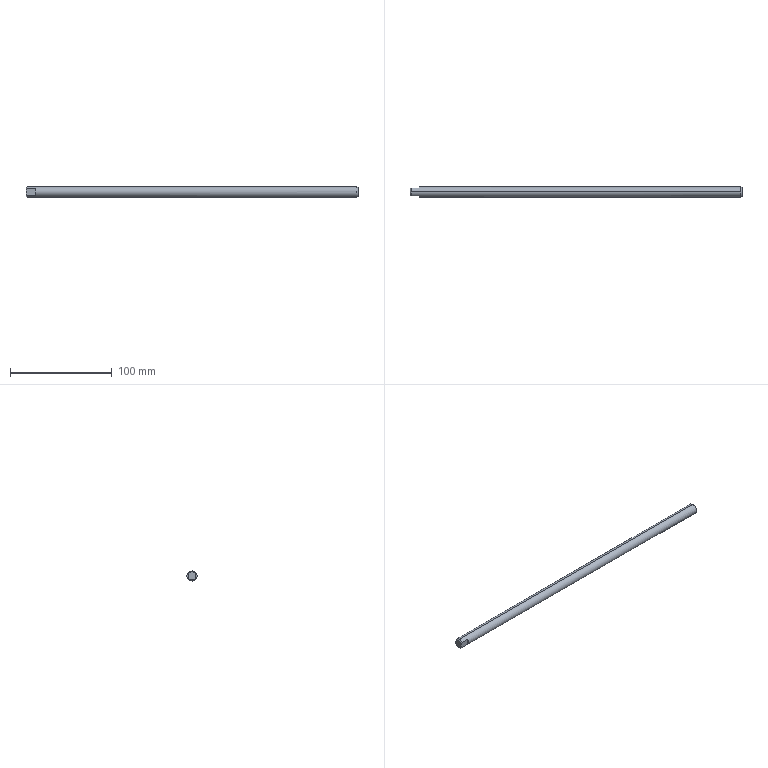Part | SolidWorks | features HoleWzd 2, Chamfer 1, Extrusion 1, ICE 1 | 1 solid | 13 faces | box 326 x 10 x 10 mm | volume 25495 mm3 | plane 6 | cone 5 | cylinder 2 | commonest cylinder face diameters 10 x2
STEP:
#1=CARTESIAN_POINT('',(326.,0.,-4.));
#2=VERTEX_POINT('',#1);
#3=CARTESIAN_POINT('',(326.,0.,4.));
#4=VERTEX_POINT('',#3);
#5=CARTESIAN_POINT('',(326.,0.,0.));
#6=DIRECTION('',(1.,0.,0.));
#7=DIRECTION('',(0.,0.,-1.));
#8=AXIS2_PLACEMENT_3D('',#5,#6,#7);
#9=CIRCLE('',#8,4.);
#10=EDGE_CURVE('',#2,#4,#9,.T.);
#11=ORIENTED_EDGE('',*,*,#10,.F.);
#12=CARTESIAN_POINT('',(325.,0.,-5.));
#13=VERTEX_POINT('',#12);
#14=CARTESIAN_POINT('',(326.,0.,-4.));
#15=DIRECTION('',(-0.7071,0.,-0.7071));
#16=VECTOR('',#15,1000.);
#17=LINE('',#14,#16);
#18=EDGE_CURVE('',#2,#13,#17,.T.);
#19=ORIENTED_EDGE('',*,*,#18,.T.);
#20=CARTESIAN_POINT('',(325.,0.,5.));
#21=VERTEX_POINT('',#20);
#22=CARTESIAN_POINT('',(325.,0.,0.));
#23=DIRECTION('',(-1.,0.,0.));
#24=DIRECTION('',(0.,0.,-1.));
#25=AXIS2_PLACEMENT_3D('',#22,#23,#24);
#26=CIRCLE('',#25,5.);
#27=EDGE_CURVE('',#21,#13,#26,.T.);
#28=ORIENTED_EDGE('',*,*,#27,.F.);
#29=CARTESIAN_POINT('',(326.,0.,4.));
#30=DIRECTION('',(-0.7071,0.,0.7071));
#31=VECTOR('',#30,1000.);
#32=LINE('',#29,#31);
#33=EDGE_CURVE('',#4,#21,#32,.T.);
#34=ORIENTED_EDGE('',*,*,#33,.F.);
#35=EDGE_LOOP('',(#11,#19,#28,#34));
#36=FACE_OUTER_BOUND('',#35,.T.);
#37=CARTESIAN_POINT('',(326.,0.,0.));
#38=DIRECTION('',(-1.,0.,0.));
#39=DIRECTION('',(0.,0.,1.));
#40=AXIS2_PLACEMENT_3D('',#37,#38,#39);
#41=CONICAL_SURFACE('',#40,4.,0.7854);
#42=ADVANCED_FACE('',(#36),#41,.T.);
#43=ORIENTED_EDGE('',*,*,#27,.T.);
#44=CARTESIAN_POINT('',(1.,0.,-5.));
#45=VERTEX_POINT('',#44);
#46=CARTESIAN_POINT('',(326.,0.,-5.));
#47=DIRECTION('',(-1.,0.,0.));
#48=VECTOR('',#47,1000.);
#49=LINE('',#46,#48);
#50=EDGE_CURVE('',#13,#45,#49,.T.);
#51=ORIENTED_EDGE('',*,*,#50,.T.);
#52=CARTESIAN_POINT('',(1.,3.9,-3.129));
#53=VERTEX_POINT('',#52);
#54=CARTESIAN_POINT('',(1.,0.,0.));
#55=DIRECTION('',(1.,0.,0.));
#56=DIRECTION('',(0.,0.,-1.));
#57=AXIS2_PLACEMENT_3D('',#54,#55,#56);
#58=CIRCLE('',#57,5.);
#59=EDGE_CURVE('',#45,#53,#58,.T.);
#60=ORIENTED_EDGE('',*,*,#59,.T.);
#61=CARTESIAN_POINT('',(9.,3.9,-3.129));
#62=VERTEX_POINT('',#61);
#63=CARTESIAN_POINT('',(326.,3.9,-3.129));
#64=DIRECTION('',(1.,0.,0.));
#65=VECTOR('',#64,1000.);
#66=LINE('',#63,#65);
#67=EDGE_CURVE('',#53,#62,#66,.T.);
#68=ORIENTED_EDGE('',*,*,#67,.T.);
#69=CARTESIAN_POINT('',(9.,3.9,3.129));
#70=VERTEX_POINT('',#69);
#71=CARTESIAN_POINT('',(9.,0.,0.));
#72=DIRECTION('',(1.,0.,0.));
#73=DIRECTION('',(0.,1.,0.));
#74=AXIS2_PLACEMENT_3D('',#71,#72,#73);
#75=CIRCLE('',#74,5.);
#76=EDGE_CURVE('',#62,#70,#75,.T.);
#77=ORIENTED_EDGE('',*,*,#76,.T.);
#78=CARTESIAN_POINT('',(1.,3.9,3.129));
#79=VERTEX_POINT('',#78);
#80=CARTESIAN_POINT('',(326.,3.9,3.129));
#81=DIRECTION('',(-1.,0.,0.));
#82=VECTOR('',#81,1000.);
#83=LINE('',#80,#82);
#84=EDGE_CURVE('',#70,#79,#83,.T.);
#85=ORIENTED_EDGE('',*,*,#84,.T.);
#86=CARTESIAN_POINT('',(1.,0.,5.));
#87=VERTEX_POINT('',#86);
#88=CARTESIAN_POINT('',(1.,0.,0.));
#89=DIRECTION('',(1.,0.,0.));
#90=DIRECTION('',(0.,0.,-1.));
#91=AXIS2_PLACEMENT_3D('',#88,#89,#90);
#92=CIRCLE('',#91,5.);
#93=EDGE_CURVE('',#79,#87,#92,.T.);
#94=ORIENTED_EDGE('',*,*,#93,.T.);
#95=CARTESIAN_POINT('',(326.,0.,5.));
#96=DIRECTION('',(-1.,0.,0.));
#97=VECTOR('',#96,1000.);
#98=LINE('',#95,#97);
#99=EDGE_CURVE('',#21,#87,#98,.T.);
#100=ORIENTED_EDGE('',*,*,#99,.F.);
#101=EDGE_LOOP('',(#43,#51,#60,#68,#77,#85,#94,#100));
#102=FACE_OUTER_BOUND('',#101,.T.);
#103=CARTESIAN_POINT('',(326.,0.,0.));
#104=DIRECTION('',(-1.,0.,0.));
#105=DIRECTION('',(0.,0.,1.));
#106=AXIS2_PLACEMENT_3D('',#103,#104,#105);
#107=CYLINDRICAL_SURFACE('',#106,5.);
#108=ADVANCED_FACE('',(#102),#107,.T.);
#109=CARTESIAN_POINT('',(0.,0.,-4.));
#110=VERTEX_POINT('',#109);
#111=CARTESIAN_POINT('',(0.,-3.9,-0.8888));
#112=VERTEX_POINT('',#111);
#113=CARTESIAN_POINT('',(0.,0.,0.));
#114=DIRECTION('',(-1.,0.,0.));
#115=DIRECTION('',(0.,0.,-1.));
#116=AXIS2_PLACEMENT_3D('',#113,#114,#115);
#117=CIRCLE('',#116,4.);
#118=EDGE_CURVE('',#110,#112,#117,.T.);
#119=ORIENTED_EDGE('',*,*,#118,.F.);
#120=CARTESIAN_POINT('',(1.,0.,-5.));
#121=DIRECTION('',(0.7071,0.,-0.7071));
#122=VECTOR('',#121,1000.);
#123=LINE('',#120,#122);
#124=EDGE_CURVE('',#110,#45,#123,.T.);
#125=ORIENTED_EDGE('',*,*,#124,.T.);
#126=CARTESIAN_POINT('',(1.,-3.9,-3.129));
#127=VERTEX_POINT('',#126);
#128=CARTESIAN_POINT('',(1.,0.,0.));
#129=DIRECTION('',(1.,0.,0.));
#130=DIRECTION('',(0.,0.,-1.));
#131=AXIS2_PLACEMENT_3D('',#128,#129,#130);
#132=CIRCLE('',#131,5.);
#133=EDGE_CURVE('',#127,#45,#132,.T.);
#134=ORIENTED_EDGE('',*,*,#133,.F.);
#135=CARTESIAN_POINT('',(0.,-3.9,-0.8888));
#136=CARTESIAN_POINT('',(0.0892,-3.9,-1.29));
#137=CARTESIAN_POINT('',(0.2351,-3.9,-1.683));
#138=CARTESIAN_POINT('',(0.5817,-3.9,-2.427));
#139=CARTESIAN_POINT('',(0.7831,-3.9,-2.782));
#140=CARTESIAN_POINT('',(1.,-3.9,-3.129));
#141=B_SPLINE_CURVE_WITH_KNOTS('',3,(#135,#136,#137,#138,#139,#140),.UNSPECIFIED.,.F.,.F.,(4,2,4),(0.01365,0.01489,0.01613),.UNSPECIFIED.);
#142=EDGE_CURVE('',#112,#127,#141,.T.);
#143=ORIENTED_EDGE('',*,*,#142,.F.);
#144=EDGE_LOOP('',(#119,#125,#134,#143));
#145=FACE_OUTER_BOUND('',#144,.T.);
#146=CARTESIAN_POINT('',(1.,0.,0.));
#147=DIRECTION('',(1.,0.,0.));
#148=DIRECTION('',(0.,0.,-1.));
#149=AXIS2_PLACEMENT_3D('',#146,#147,#148);
#150=CONICAL_SURFACE('',#149,5.,0.7854);
#151=ADVANCED_FACE('',(#145),#150,.T.);
#152=ORIENTED_EDGE('',*,*,#124,.F.);
#153=CARTESIAN_POINT('',(0.,3.9,-0.8888));
#154=VERTEX_POINT('',#153);
#155=CARTESIAN_POINT('',(0.,0.,0.));
#156=DIRECTION('',(-1.,0.,0.));
#157=DIRECTION('',(0.,0.,-1.));
#158=AXIS2_PLACEMENT_3D('',#155,#156,#157);
#159=CIRCLE('',#158,4.);
#160=EDGE_CURVE('',#154,#110,#159,.T.);
#161=ORIENTED_EDGE('',*,*,#160,.F.);
#162=CARTESIAN_POINT('',(1.,3.9,-3.129));
#163=CARTESIAN_POINT('',(0.7819,3.9,-2.78));
#164=CARTESIAN_POINT('',(0.579,3.9,-2.422));
#165=CARTESIAN_POINT('',(0.3197,3.9,-1.865));
#166=CARTESIAN_POINT('',(0.2407,3.9,-1.675));
#167=CARTESIAN_POINT('',(0.1029,3.9,-1.287));
#168=CARTESIAN_POINT('',(0.04437,3.9,-1.088));
#169=CARTESIAN_POINT('',(0.,3.9,-0.8888));
#170=B_SPLINE_CURVE_WITH_KNOTS('',3,(#162,#163,#164,#165,#166,#167,#168,#169),.UNSPECIFIED.,.F.,.F.,(4,2,2,4),(0.009397,0.01063,0.01124,0.01186),.UNSPECIFIED.);
#171=EDGE_CURVE('',#53,#154,#170,.T.);
#172=ORIENTED_EDGE('',*,*,#171,.F.);
#173=ORIENTED_EDGE('',*,*,#59,.F.);
#174=EDGE_LOOP('',(#152,#161,#172,#173));
#175=FACE_OUTER_BOUND('',#174,.T.);
#176=CARTESIAN_POINT('',(1.,0.,0.));
#177=DIRECTION('',(1.,0.,0.));
#178=DIRECTION('',(0.,0.,-1.));
#179=AXIS2_PLACEMENT_3D('',#176,#177,#178);
#180=CONICAL_SURFACE('',#179,5.,0.7854);
#181=ADVANCED_FACE('',(#175),#180,.T.);
#182=ORIENTED_EDGE('',*,*,#50,.F.);
#183=CARTESIAN_POINT('',(325.,0.,0.));
#184=DIRECTION('',(-1.,0.,0.));
#185=DIRECTION('',(0.,0.,-1.));
#186=AXIS2_PLACEMENT_3D('',#183,#184,#185);
#187=CIRCLE('',#186,5.);
#188=EDGE_CURVE('',#13,#21,#187,.T.);
#189=ORIENTED_EDGE('',*,*,#188,.T.);
#190=ORIENTED_EDGE('',*,*,#99,.T.);
#191=CARTESIAN_POINT('',(1.,-3.9,3.129));
#192=VERTEX_POINT('',#191);
#193=CARTESIAN_POINT('',(1.,0.,0.));
#194=DIRECTION('',(1.,0.,0.));
#195=DIRECTION('',(0.,0.,-1.));
#196=AXIS2_PLACEMENT_3D('',#193,#194,#195);
#197=CIRCLE('',#196,5.);
#198=EDGE_CURVE('',#87,#192,#197,.T.);
#199=ORIENTED_EDGE('',*,*,#198,.T.);
#200=CARTESIAN_POINT('',(9.,-3.9,3.129));
#201=VERTEX_POINT('',#200);
#202=CARTESIAN_POINT('',(326.,-3.9,3.129));
#203=DIRECTION('',(1.,0.,0.));
#204=VECTOR('',#203,1000.);
#205=LINE('',#202,#204);
#206=EDGE_CURVE('',#192,#201,#205,.T.);
#207=ORIENTED_EDGE('',*,*,#206,.T.);
#208=CARTESIAN_POINT('',(9.,-3.9,-3.129));
#209=VERTEX_POINT('',#208);
#210=CARTESIAN_POINT('',(9.,0.,0.));
#211=DIRECTION('',(1.,0.,0.));
#212=DIRECTION('',(0.,1.,0.));
#213=AXIS2_PLACEMENT_3D('',#210,#211,#212);
#214=CIRCLE('',#213,5.);
#215=EDGE_CURVE('',#201,#209,#214,.T.);
#216=ORIENTED_EDGE('',*,*,#215,.T.);
#217=CARTESIAN_POINT('',(326.,-3.9,-3.129));
#218=DIRECTION('',(-1.,0.,0.));
#219=VECTOR('',#218,1000.);
#220=LINE('',#217,#219);
#221=EDGE_CURVE('',#209,#127,#220,.T.);
#222=ORIENTED_EDGE('',*,*,#221,.T.);
#223=ORIENTED_EDGE('',*,*,#133,.T.);
#224=EDGE_LOOP('',(#182,#189,#190,#199,#207,#216,#222,#223));
#225=FACE_OUTER_BOUND('',#224,.T.);
#226=CARTESIAN_POINT('',(326.,0.,0.));
#227=DIRECTION('',(-1.,0.,0.));
#228=DIRECTION('',(0.,0.,1.));
#229=AXIS2_PLACEMENT_3D('',#226,#227,#228);
#230=CYLINDRICAL_SURFACE('',#229,5.);
#231=ADVANCED_FACE('',(#225),#230,.T.);
#232=CARTESIAN_POINT('',(326.,0.,0.));
#233=DIRECTION('',(1.,0.,0.));
#234=DIRECTION('',(0.,0.,-1.));
#235=AXIS2_PLACEMENT_3D('',#232,#233,#234);
#236=CIRCLE('',#235,4.);
#237=EDGE_CURVE('',#4,#2,#236,.T.);
#238=ORIENTED_EDGE('',*,*,#237,.T.);
#239=ORIENTED_EDGE('',*,*,#10,.T.);
#240=EDGE_LOOP('',(#238,#239));
#241=FACE_OUTER_BOUND('',#240,.T.);
#242=CARTESIAN_POINT('',(326.,0.,0.));
#243=DIRECTION('',(1.,0.,0.));
#244=DIRECTION('',(0.,0.,-1.));
#245=AXIS2_PLACEMENT_3D('',#242,#243,#244);
#246=PLANE('',#245);
#247=ADVANCED_FACE('',(#241),#246,.T.);
#248=CARTESIAN_POINT('',(0.,-3.9,0.8888));
#249=VERTEX_POINT('',#248);
#250=CARTESIAN_POINT('',(0.,3.9,0.8888));
#251=VERTEX_POINT('',#250);
#252=CARTESIAN_POINT('',(0.,0.,0.));
#253=DIRECTION('',(-1.,0.,0.));
#254=DIRECTION('',(0.,0.,-1.));
#255=AXIS2_PLACEMENT_3D('',#252,#253,#254);
#256=CIRCLE('',#255,4.);
#257=EDGE_CURVE('',#249,#251,#256,.T.);
#258=ORIENTED_EDGE('',*,*,#257,.T.);
#259=CARTESIAN_POINT('',(0.,3.9,0.));
#260=DIRECTION('',(0.,0.,-1.));
#261=VECTOR('',#260,1000.);
#262=LINE('',#259,#261);
#263=EDGE_CURVE('',#251,#154,#262,.T.);
#264=ORIENTED_EDGE('',*,*,#263,.T.);
#265=ORIENTED_EDGE('',*,*,#160,.T.);
#266=ORIENTED_EDGE('',*,*,#118,.T.);
#267=CARTESIAN_POINT('',(0.,-3.9,0.));
#268=DIRECTION('',(0.,0.,1.));
#269=VECTOR('',#268,1000.);
#270=LINE('',#267,#269);
#271=EDGE_CURVE('',#112,#249,#270,.T.);
#272=ORIENTED_EDGE('',*,*,#271,.T.);
#273=EDGE_LOOP('',(#258,#264,#265,#266,#272));
#274=FACE_OUTER_BOUND('',#273,.T.);
#275=CARTESIAN_POINT('',(0.,0.,0.));
#276=DIRECTION('',(1.,0.,0.));
#277=DIRECTION('',(0.,0.,-1.));
#278=AXIS2_PLACEMENT_3D('',#275,#276,#277);
#279=PLANE('',#278);
#280=ADVANCED_FACE('',(#274),#279,.F.);
#281=CARTESIAN_POINT('',(0.,3.9,0.8888));
#282=CARTESIAN_POINT('',(0.0892,3.9,1.29));
#283=CARTESIAN_POINT('',(0.2351,3.9,1.683));
#284=CARTESIAN_POINT('',(0.5817,3.9,2.427));
#285=CARTESIAN_POINT('',(0.7831,3.9,2.782));
#286=CARTESIAN_POINT('',(1.,3.9,3.129));
#287=B_SPLINE_CURVE_WITH_KNOTS('',3,(#281,#282,#283,#284,#285,#286),.UNSPECIFIED.,.F.,.F.,(4,2,4),(0.01365,0.01489,0.01613),.UNSPECIFIED.);
#288=EDGE_CURVE('',#251,#79,#287,.T.);
#289=ORIENTED_EDGE('',*,*,#288,.F.);
#290=ORIENTED_EDGE('',*,*,#257,.F.);
#291=CARTESIAN_POINT('',(1.,-3.9,3.129));
#292=CARTESIAN_POINT('',(0.7819,-3.9,2.78));
#293=CARTESIAN_POINT('',(0.579,-3.9,2.422));
#294=CARTESIAN_POINT('',(0.3197,-3.9,1.865));
#295=CARTESIAN_POINT('',(0.2407,-3.9,1.675));
#296=CARTESIAN_POINT('',(0.1029,-3.9,1.287));
#297=CARTESIAN_POINT('',(0.04437,-3.9,1.088));
#298=CARTESIAN_POINT('',(0.,-3.9,0.8888));
#299=B_SPLINE_CURVE_WITH_KNOTS('',3,(#291,#292,#293,#294,#295,#296,#297,#298),.UNSPECIFIED.,.F.,.F.,(4,2,2,4),(0.009397,0.01063,0.01124,0.01186),.UNSPECIFIED.);
#300=EDGE_CURVE('',#192,#249,#299,.T.);
#301=ORIENTED_EDGE('',*,*,#300,.F.);
#302=ORIENTED_EDGE('',*,*,#198,.F.);
#303=ORIENTED_EDGE('',*,*,#93,.F.);
#304=EDGE_LOOP('',(#289,#290,#301,#302,#303));
#305=FACE_OUTER_BOUND('',#304,.T.);
#306=CARTESIAN_POINT('',(1.,0.,0.));
#307=DIRECTION('',(1.,0.,0.));
#308=DIRECTION('',(0.,0.,-1.));
#309=AXIS2_PLACEMENT_3D('',#306,#307,#308);
#310=CONICAL_SURFACE('',#309,5.,0.7854);
#311=ADVANCED_FACE('',(#305),#310,.T.);
#312=ORIENTED_EDGE('',*,*,#18,.F.);
#313=ORIENTED_EDGE('',*,*,#237,.F.);
#314=ORIENTED_EDGE('',*,*,#33,.T.);
#315=ORIENTED_EDGE('',*,*,#188,.F.);
#316=EDGE_LOOP('',(#312,#313,#314,#315));
#317=FACE_OUTER_BOUND('',#316,.T.);
#318=CARTESIAN_POINT('',(326.,0.,0.));
#319=DIRECTION('',(-1.,0.,0.));
#320=DIRECTION('',(0.,0.,1.));
#321=AXIS2_PLACEMENT_3D('',#318,#319,#320);
#322=CONICAL_SURFACE('',#321,4.,0.7854);
#323=ADVANCED_FACE('',(#317),#322,.T.);
#324=CARTESIAN_POINT('',(9.,-3.9,-5.));
#325=DIRECTION('',(0.,0.,1.));
#326=VECTOR('',#325,1000.);
#327=LINE('',#324,#326);
#328=EDGE_CURVE('',#209,#201,#327,.T.);
#329=ORIENTED_EDGE('',*,*,#328,.F.);
#330=ORIENTED_EDGE('',*,*,#215,.F.);
#331=EDGE_LOOP('',(#329,#330));
#332=FACE_OUTER_BOUND('',#331,.T.);
#333=CARTESIAN_POINT('',(9.,-11.476,-5.));
#334=DIRECTION('',(1.,0.,0.));
#335=DIRECTION('',(0.,1.,0.));
#336=AXIS2_PLACEMENT_3D('',#333,#334,#335);
#337=PLANE('',#336);
#338=ADVANCED_FACE('',(#332),#337,.F.);
#339=ORIENTED_EDGE('',*,*,#300,.T.);
#340=ORIENTED_EDGE('',*,*,#271,.F.);
#341=ORIENTED_EDGE('',*,*,#142,.T.);
#342=ORIENTED_EDGE('',*,*,#221,.F.);
#343=ORIENTED_EDGE('',*,*,#328,.T.);
#344=ORIENTED_EDGE('',*,*,#206,.F.);
#345=EDGE_LOOP('',(#339,#340,#341,#342,#343,#344));
#346=FACE_OUTER_BOUND('',#345,.T.);
#347=CARTESIAN_POINT('',(-147.813,-3.9,-5.));
#348=DIRECTION('',(0.,1.,0.));
#349=DIRECTION('',(0.,0.,1.));
#350=AXIS2_PLACEMENT_3D('',#347,#348,#349);
#351=PLANE('',#350);
#352=ADVANCED_FACE('',(#346),#351,.F.);
#353=CARTESIAN_POINT('',(9.,3.9,-5.));
#354=DIRECTION('',(0.,0.,1.));
#355=VECTOR('',#354,1000.);
#356=LINE('',#353,#355);
#357=EDGE_CURVE('',#62,#70,#356,.T.);
#358=ORIENTED_EDGE('',*,*,#357,.T.);
#359=ORIENTED_EDGE('',*,*,#76,.F.);
#360=EDGE_LOOP('',(#358,#359));
#361=FACE_OUTER_BOUND('',#360,.T.);
#362=CARTESIAN_POINT('',(9.,11.476,-5.));
#363=DIRECTION('',(1.,0.,0.));
#364=DIRECTION('',(0.,1.,0.));
#365=AXIS2_PLACEMENT_3D('',#362,#363,#364);
#366=PLANE('',#365);
#367=ADVANCED_FACE('',(#361),#366,.F.);
#368=ORIENTED_EDGE('',*,*,#171,.T.);
#369=ORIENTED_EDGE('',*,*,#263,.F.);
#370=ORIENTED_EDGE('',*,*,#288,.T.);
#371=ORIENTED_EDGE('',*,*,#84,.F.);
#372=ORIENTED_EDGE('',*,*,#357,.F.);
#373=ORIENTED_EDGE('',*,*,#67,.F.);
#374=EDGE_LOOP('',(#368,#369,#370,#371,#372,#373));
#375=FACE_OUTER_BOUND('',#374,.T.);
#376=CARTESIAN_POINT('',(-147.813,3.9,-5.));
#377=DIRECTION('',(0.,-1.,0.));
#378=DIRECTION('',(0.,0.,-1.));
#379=AXIS2_PLACEMENT_3D('',#376,#377,#378);
#380=PLANE('',#379);
#381=ADVANCED_FACE('',(#375),#380,.F.);
#382=CLOSED_SHELL('',(#42,#108,#151,#181,#231,#247,#280,#311,#323,#338,#352,#367,#381));
#383=MANIFOLD_SOLID_BREP('',#382);
#384=CARTESIAN_POINT('',(0.,0.,0.));
#385=DIRECTION('',(0.,0.,1.));
#386=DIRECTION('',(1.,0.,0.));
#387=AXIS2_PLACEMENT_3D('',#384,#385,#386);
#388=(LENGTH_UNIT()NAMED_UNIT(*)SI_UNIT(.MILLI.,.METRE.));
#389=UNCERTAINTY_MEASURE_WITH_UNIT(LENGTH_MEASURE(0.00001),#388,'','');
#390=(NAMED_UNIT(*)PLANE_ANGLE_UNIT()SI_UNIT($,.RADIAN.));
#391=(NAMED_UNIT(*)SI_UNIT($,.STERADIAN.)SOLID_ANGLE_UNIT());
#392=(GEOMETRIC_REPRESENTATION_CONTEXT(3)GLOBAL_UNCERTAINTY_ASSIGNED_CONTEXT((#389))GLOBAL_UNIT_ASSIGNED_CONTEXT((#388,#390,#391))REPRESENTATION_CONTEXT('',''));
#393=ADVANCED_BREP_SHAPE_REPRESENTATION('',(#383,#387),#392);